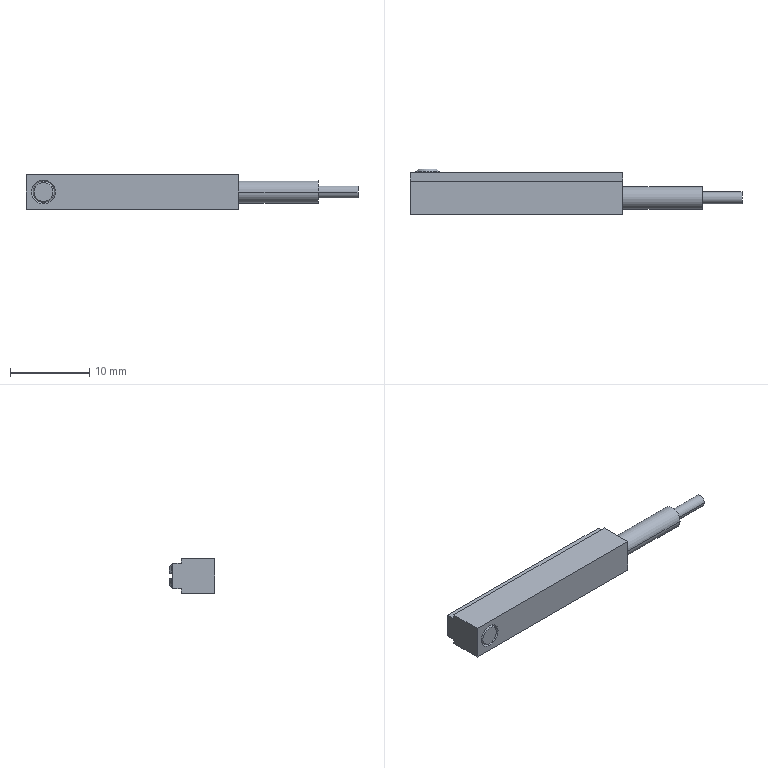Part | SolidWorks | features BaseBody 1 | 1 solid | 34 faces | box 41.8 x 5.7 x 4.4 mm | volume 661.389 mm3 | plane 20 | cylinder 7 | cone 7 | commonest cylinder face diameters 3 x3 1.5 x2 2.8 x2
STEP:
#1=CARTESIAN_POINT('',(2.2,3.2,-1.5));
#2=VERTEX_POINT('',#1);
#3=CARTESIAN_POINT('',(3.67,3.2,-0.3));
#4=VERTEX_POINT('',#3);
#5=CARTESIAN_POINT('',(2.2,3.2,0.));
#6=DIRECTION('',(0.,-1.,0.));
#7=DIRECTION('',(1.,0.,0.));
#8=AXIS2_PLACEMENT_3D('',#5,#6,#7);
#9=CIRCLE('',#8,1.5);
#10=EDGE_CURVE('',#2,#4,#9,.T.);
#11=ORIENTED_EDGE('',*,*,#10,.F.);
#12=CARTESIAN_POINT('',(2.2,3.293,-1.5));
#13=VERTEX_POINT('',#12);
#14=CARTESIAN_POINT('',(2.2,-2.1,-1.5));
#15=DIRECTION('',(0.,1.,0.));
#16=VECTOR('',#15,1000.);
#17=LINE('',#14,#16);
#18=EDGE_CURVE('',#2,#13,#17,.T.);
#19=ORIENTED_EDGE('',*,*,#18,.T.);
#20=CARTESIAN_POINT('',(3.67,3.293,-0.3));
#21=VERTEX_POINT('',#20);
#22=CARTESIAN_POINT('',(2.2,3.293,0.));
#23=DIRECTION('',(0.,-1.,0.));
#24=DIRECTION('',(0.,0.,-1.));
#25=AXIS2_PLACEMENT_3D('',#22,#23,#24);
#26=CIRCLE('',#25,1.5);
#27=EDGE_CURVE('',#13,#21,#26,.T.);
#28=ORIENTED_EDGE('',*,*,#27,.T.);
#29=CARTESIAN_POINT('',(3.67,-2.1,-0.3));
#30=DIRECTION('',(0.,1.,0.));
#31=VECTOR('',#30,1000.);
#32=LINE('',#29,#31);
#33=EDGE_CURVE('',#4,#21,#32,.T.);
#34=ORIENTED_EDGE('',*,*,#33,.F.);
#35=EDGE_LOOP('',(#11,#19,#28,#34));
#36=FACE_OUTER_BOUND('',#35,.T.);
#37=CARTESIAN_POINT('',(2.2,-2.1,0.));
#38=DIRECTION('',(0.,1.,0.));
#39=DIRECTION('',(0.,0.,-1.));
#40=AXIS2_PLACEMENT_3D('',#37,#38,#39);
#41=CYLINDRICAL_SURFACE('',#40,1.5);
#42=ADVANCED_FACE('',(#36),#41,.T.);
#43=CARTESIAN_POINT('',(1.045,3.6,-0.3));
#44=VERTEX_POINT('',#43);
#45=CARTESIAN_POINT('',(2.2,3.6,-1.194));
#46=VERTEX_POINT('',#45);
#47=CARTESIAN_POINT('',(2.2,3.6,0.));
#48=DIRECTION('',(0.,-1.,0.));
#49=DIRECTION('',(0.,0.,-1.));
#50=AXIS2_PLACEMENT_3D('',#47,#48,#49);
#51=CIRCLE('',#50,1.194);
#52=EDGE_CURVE('',#44,#46,#51,.T.);
#53=ORIENTED_EDGE('',*,*,#52,.T.);
#54=CARTESIAN_POINT('',(2.2,3.6,-1.194));
#55=DIRECTION('',(0.,-0.7071,-0.7071));
#56=VECTOR('',#55,1000.);
#57=LINE('',#54,#56);
#58=EDGE_CURVE('',#46,#13,#57,.T.);
#59=ORIENTED_EDGE('',*,*,#58,.T.);
#60=CARTESIAN_POINT('',(0.7303,3.293,-0.3));
#61=VERTEX_POINT('',#60);
#62=CARTESIAN_POINT('',(2.2,3.293,0.));
#63=DIRECTION('',(0.,-1.,0.));
#64=DIRECTION('',(0.,0.,-1.));
#65=AXIS2_PLACEMENT_3D('',#62,#63,#64);
#66=CIRCLE('',#65,1.5);
#67=EDGE_CURVE('',#61,#13,#66,.T.);
#68=ORIENTED_EDGE('',*,*,#67,.F.);
#69=CARTESIAN_POINT('',(1.045,3.6,-0.3));
#70=CARTESIAN_POINT('',(0.9396,3.498,-0.3));
#71=CARTESIAN_POINT('',(0.8349,3.396,-0.3));
#72=CARTESIAN_POINT('',(0.7303,3.293,-0.3));
#73=B_SPLINE_CURVE_WITH_KNOTS('',3,(#69,#70,#71,#72),.UNSPECIFIED.,.F.,.F.,(4,4),(0.005968,0.006407),.UNSPECIFIED.);
#74=EDGE_CURVE('',#44,#61,#73,.T.);
#75=ORIENTED_EDGE('',*,*,#74,.F.);
#76=EDGE_LOOP('',(#53,#59,#68,#75));
#77=FACE_OUTER_BOUND('',#76,.T.);
#78=CARTESIAN_POINT('',(2.2,3.6,0.));
#79=DIRECTION('',(0.,-1.,0.));
#80=DIRECTION('',(0.,0.,-1.));
#81=AXIS2_PLACEMENT_3D('',#78,#79,#80);
#82=CONICAL_SURFACE('',#81,1.194,0.7854);
#83=ADVANCED_FACE('',(#77),#82,.T.);
#84=CARTESIAN_POINT('',(36.8,-1.4,0.));
#85=VERTEX_POINT('',#84);
#86=CARTESIAN_POINT('',(36.8,1.4,0.));
#87=VERTEX_POINT('',#86);
#88=CARTESIAN_POINT('',(36.8,0.,0.));
#89=DIRECTION('',(1.,0.,0.));
#90=DIRECTION('',(0.,1.,0.));
#91=AXIS2_PLACEMENT_3D('',#88,#89,#90);
#92=CIRCLE('',#91,1.4);
#93=EDGE_CURVE('',#85,#87,#92,.T.);
#94=ORIENTED_EDGE('',*,*,#93,.F.);
#95=CARTESIAN_POINT('',(26.8,-1.4,0.));
#96=VERTEX_POINT('',#95);
#97=CARTESIAN_POINT('',(41.8,-1.4,0.));
#98=DIRECTION('',(-1.,0.,0.));
#99=VECTOR('',#98,1000.);
#100=LINE('',#97,#99);
#101=EDGE_CURVE('',#85,#96,#100,.T.);
#102=ORIENTED_EDGE('',*,*,#101,.T.);
#103=CARTESIAN_POINT('',(26.8,1.4,0.));
#104=VERTEX_POINT('',#103);
#105=CARTESIAN_POINT('',(26.8,0.,0.));
#106=DIRECTION('',(1.,0.,0.));
#107=DIRECTION('',(0.,1.,0.));
#108=AXIS2_PLACEMENT_3D('',#105,#106,#107);
#109=CIRCLE('',#108,1.4);
#110=EDGE_CURVE('',#96,#104,#109,.T.);
#111=ORIENTED_EDGE('',*,*,#110,.T.);
#112=CARTESIAN_POINT('',(41.8,1.4,0.));
#113=DIRECTION('',(-1.,0.,0.));
#114=VECTOR('',#113,1000.);
#115=LINE('',#112,#114);
#116=EDGE_CURVE('',#87,#104,#115,.T.);
#117=ORIENTED_EDGE('',*,*,#116,.F.);
#118=EDGE_LOOP('',(#94,#102,#111,#117));
#119=FACE_OUTER_BOUND('',#118,.T.);
#120=CARTESIAN_POINT('',(41.8,0.,0.));
#121=DIRECTION('',(-1.,0.,0.));
#122=DIRECTION('',(0.,1.,0.));
#123=AXIS2_PLACEMENT_3D('',#120,#121,#122);
#124=CYLINDRICAL_SURFACE('',#123,1.4);
#125=ADVANCED_FACE('',(#119),#124,.T.);
#126=CARTESIAN_POINT('',(41.8,-0.75,0.));
#127=VERTEX_POINT('',#126);
#128=CARTESIAN_POINT('',(41.8,0.75,0.));
#129=VERTEX_POINT('',#128);
#130=CARTESIAN_POINT('',(41.8,0.,0.));
#131=DIRECTION('',(1.,0.,0.));
#132=DIRECTION('',(0.,1.,0.));
#133=AXIS2_PLACEMENT_3D('',#130,#131,#132);
#134=CIRCLE('',#133,0.75);
#135=EDGE_CURVE('',#127,#129,#134,.T.);
#136=ORIENTED_EDGE('',*,*,#135,.F.);
#137=CARTESIAN_POINT('',(36.8,-0.75,0.));
#138=VERTEX_POINT('',#137);
#139=CARTESIAN_POINT('',(41.8,-0.75,0.));
#140=DIRECTION('',(-1.,0.,0.));
#141=VECTOR('',#140,1000.);
#142=LINE('',#139,#141);
#143=EDGE_CURVE('',#127,#138,#142,.T.);
#144=ORIENTED_EDGE('',*,*,#143,.T.);
#145=CARTESIAN_POINT('',(36.8,0.75,0.));
#146=VERTEX_POINT('',#145);
#147=CARTESIAN_POINT('',(36.8,0.,0.));
#148=DIRECTION('',(1.,0.,0.));
#149=DIRECTION('',(0.,1.,0.));
#150=AXIS2_PLACEMENT_3D('',#147,#148,#149);
#151=CIRCLE('',#150,0.75);
#152=EDGE_CURVE('',#138,#146,#151,.T.);
#153=ORIENTED_EDGE('',*,*,#152,.T.);
#154=CARTESIAN_POINT('',(41.8,0.75,0.));
#155=DIRECTION('',(-1.,0.,0.));
#156=VECTOR('',#155,1000.);
#157=LINE('',#154,#156);
#158=EDGE_CURVE('',#129,#146,#157,.T.);
#159=ORIENTED_EDGE('',*,*,#158,.F.);
#160=EDGE_LOOP('',(#136,#144,#153,#159));
#161=FACE_OUTER_BOUND('',#160,.T.);
#162=CARTESIAN_POINT('',(41.8,0.,0.));
#163=DIRECTION('',(-1.,0.,0.));
#164=DIRECTION('',(0.,1.,0.));
#165=AXIS2_PLACEMENT_3D('',#162,#163,#164);
#166=CYLINDRICAL_SURFACE('',#165,0.75);
#167=ADVANCED_FACE('',(#161),#166,.T.);
#168=CARTESIAN_POINT('',(2.2,-2.1,-1.194));
#169=VERTEX_POINT('',#168);
#170=CARTESIAN_POINT('',(2.2,-2.1,1.194));
#171=VERTEX_POINT('',#170);
#172=CARTESIAN_POINT('',(2.2,-2.1,0.));
#173=DIRECTION('',(0.,-1.,0.));
#174=DIRECTION('',(0.,0.,-1.));
#175=AXIS2_PLACEMENT_3D('',#172,#173,#174);
#176=CIRCLE('',#175,1.194);
#177=EDGE_CURVE('',#169,#171,#176,.T.);
#178=ORIENTED_EDGE('',*,*,#177,.F.);
#179=CARTESIAN_POINT('',(2.2,-1.947,-1.347));
#180=VERTEX_POINT('',#179);
#181=CARTESIAN_POINT('',(2.2,-1.793,-1.5));
#182=DIRECTION('',(0.,0.7071,-0.7071));
#183=VECTOR('',#182,1000.);
#184=LINE('',#181,#183);
#185=EDGE_CURVE('',#169,#180,#184,.T.);
#186=ORIENTED_EDGE('',*,*,#185,.T.);
#187=CARTESIAN_POINT('',(3.547,-1.947,0.));
#188=VERTEX_POINT('',#187);
#189=CARTESIAN_POINT('',(2.2,-1.947,0.));
#190=DIRECTION('',(0.,1.,0.));
#191=DIRECTION('',(0.,0.,1.));
#192=AXIS2_PLACEMENT_3D('',#189,#190,#191);
#193=CIRCLE('',#192,1.347);
#194=EDGE_CURVE('',#188,#180,#193,.T.);
#195=ORIENTED_EDGE('',*,*,#194,.F.);
#196=CARTESIAN_POINT('',(2.2,-1.947,1.347));
#197=VERTEX_POINT('',#196);
#198=CARTESIAN_POINT('',(2.2,-1.947,0.));
#199=DIRECTION('',(0.,1.,0.));
#200=DIRECTION('',(0.,0.,1.));
#201=AXIS2_PLACEMENT_3D('',#198,#199,#200);
#202=CIRCLE('',#201,1.347);
#203=EDGE_CURVE('',#197,#188,#202,.T.);
#204=ORIENTED_EDGE('',*,*,#203,.F.);
#205=CARTESIAN_POINT('',(2.2,-1.793,1.5));
#206=DIRECTION('',(0.,0.7071,0.7071));
#207=VECTOR('',#206,1000.);
#208=LINE('',#205,#207);
#209=EDGE_CURVE('',#171,#197,#208,.T.);
#210=ORIENTED_EDGE('',*,*,#209,.F.);
#211=EDGE_LOOP('',(#178,#186,#195,#204,#210));
#212=FACE_OUTER_BOUND('',#211,.T.);
#213=CARTESIAN_POINT('',(2.2,-1.793,0.));
#214=DIRECTION('',(0.,1.,0.));
#215=DIRECTION('',(0.,0.,1.));
#216=AXIS2_PLACEMENT_3D('',#213,#214,#215);
#217=CONICAL_SURFACE('',#216,1.5,0.7854);
#218=ADVANCED_FACE('',(#212),#217,.T.);
#219=ORIENTED_EDGE('',*,*,#194,.T.);
#220=CARTESIAN_POINT('',(0.8533,-1.947,0.));
#221=VERTEX_POINT('',#220);
#222=CARTESIAN_POINT('',(2.2,-1.947,0.));
#223=DIRECTION('',(0.,1.,0.));
#224=DIRECTION('',(0.,0.,1.));
#225=AXIS2_PLACEMENT_3D('',#222,#223,#224);
#226=CIRCLE('',#225,1.347);
#227=EDGE_CURVE('',#180,#221,#226,.T.);
#228=ORIENTED_EDGE('',*,*,#227,.T.);
#229=CARTESIAN_POINT('',(0.7,-2.1,0.));
#230=VERTEX_POINT('',#229);
#231=CARTESIAN_POINT('',(0.9705,-1.83,0.));
#232=DIRECTION('',(-0.7071,-0.7071,0.));
#233=VECTOR('',#232,1000.);
#234=LINE('',#231,#233);
#235=EDGE_CURVE('',#221,#230,#234,.T.);
#236=ORIENTED_EDGE('',*,*,#235,.T.);
#237=CARTESIAN_POINT('',(3.7,-2.1,0.));
#238=VERTEX_POINT('',#237);
#239=CARTESIAN_POINT('',(2.2,-2.1,0.));
#240=DIRECTION('',(0.,-1.,0.));
#241=DIRECTION('',(1.,0.,0.));
#242=AXIS2_PLACEMENT_3D('',#239,#240,#241);
#243=CIRCLE('',#242,1.5);
#244=EDGE_CURVE('',#230,#238,#243,.T.);
#245=ORIENTED_EDGE('',*,*,#244,.T.);
#246=CARTESIAN_POINT('',(3.43,-1.829,0.));
#247=DIRECTION('',(0.7071,-0.7071,0.));
#248=VECTOR('',#247,1000.);
#249=LINE('',#246,#248);
#250=EDGE_CURVE('',#188,#238,#249,.T.);
#251=ORIENTED_EDGE('',*,*,#250,.F.);
#252=EDGE_LOOP('',(#219,#228,#236,#245,#251));
#253=FACE_OUTER_BOUND('',#252,.T.);
#254=CARTESIAN_POINT('',(2.2,-1.829,0.));
#255=DIRECTION('',(0.,-1.,0.));
#256=DIRECTION('',(1.,0.,0.));
#257=AXIS2_PLACEMENT_3D('',#254,#255,#256);
#258=CONICAL_SURFACE('',#257,1.23,0.7854);
#259=ADVANCED_FACE('',(#253),#258,.F.);
#260=CARTESIAN_POINT('',(0.,-2.1,-2.2));
#261=VERTEX_POINT('',#260);
#262=CARTESIAN_POINT('',(0.,2.1,-2.2));
#263=VERTEX_POINT('',#262);
#264=CARTESIAN_POINT('',(0.,-2.1,-2.2));
#265=DIRECTION('',(0.,1.,0.));
#266=VECTOR('',#265,1000.);
#267=LINE('',#264,#266);
#268=EDGE_CURVE('',#261,#263,#267,.T.);
#269=ORIENTED_EDGE('',*,*,#268,.T.);
#270=CARTESIAN_POINT('',(26.8,2.1,-2.2));
#271=VERTEX_POINT('',#270);
#272=CARTESIAN_POINT('',(26.8,2.1,-2.2));
#273=DIRECTION('',(-1.,0.,0.));
#274=VECTOR('',#273,1000.);
#275=LINE('',#272,#274);
#276=EDGE_CURVE('',#271,#263,#275,.T.);
#277=ORIENTED_EDGE('',*,*,#276,.F.);
#278=CARTESIAN_POINT('',(26.8,-2.1,-2.2));
#279=VERTEX_POINT('',#278);
#280=CARTESIAN_POINT('',(26.8,-2.1,-2.2));
#281=DIRECTION('',(0.,1.,0.));
#282=VECTOR('',#281,1000.);
#283=LINE('',#280,#282);
#284=EDGE_CURVE('',#279,#271,#283,.T.);
#285=ORIENTED_EDGE('',*,*,#284,.F.);
#286=CARTESIAN_POINT('',(26.8,-2.1,-2.2));
#287=DIRECTION('',(-1.,0.,0.));
#288=VECTOR('',#287,1000.);
#289=LINE('',#286,#288);
#290=EDGE_CURVE('',#279,#261,#289,.T.);
#291=ORIENTED_EDGE('',*,*,#290,.T.);
#292=EDGE_LOOP('',(#269,#277,#285,#291));
#293=FACE_OUTER_BOUND('',#292,.T.);
#294=CARTESIAN_POINT('',(26.8,-2.1,-2.2));
#295=DIRECTION('',(0.,0.,1.));
#296=DIRECTION('',(1.,0.,0.));
#297=AXIS2_PLACEMENT_3D('',#294,#295,#296);
#298=PLANE('',#297);
#299=ADVANCED_FACE('',(#293),#298,.F.);
#300=CARTESIAN_POINT('',(0.,2.1,-1.6));
#301=VERTEX_POINT('',#300);
#302=CARTESIAN_POINT('',(0.,2.1,-2.2));
#303=DIRECTION('',(0.,0.,1.));
#304=VECTOR('',#303,1000.);
#305=LINE('',#302,#304);
#306=EDGE_CURVE('',#263,#301,#305,.T.);
#307=ORIENTED_EDGE('',*,*,#306,.T.);
#308=CARTESIAN_POINT('',(26.8,2.1,-1.6));
#309=VERTEX_POINT('',#308);
#310=CARTESIAN_POINT('',(26.8,2.1,-1.6));
#311=DIRECTION('',(-1.,0.,0.));
#312=VECTOR('',#311,1000.);
#313=LINE('',#310,#312);
#314=EDGE_CURVE('',#309,#301,#313,.T.);
#315=ORIENTED_EDGE('',*,*,#314,.F.);
#316=CARTESIAN_POINT('',(26.8,2.1,-2.2));
#317=DIRECTION('',(0.,0.,1.));
#318=VECTOR('',#317,1000.);
#319=LINE('',#316,#318);
#320=EDGE_CURVE('',#271,#309,#319,.T.);
#321=ORIENTED_EDGE('',*,*,#320,.F.);
#322=ORIENTED_EDGE('',*,*,#276,.T.);
#323=EDGE_LOOP('',(#307,#315,#321,#322));
#324=FACE_OUTER_BOUND('',#323,.T.);
#325=CARTESIAN_POINT('',(26.8,2.1,-2.2));
#326=DIRECTION('',(0.,-1.,0.));
#327=DIRECTION('',(0.,0.,-1.));
#328=AXIS2_PLACEMENT_3D('',#325,#326,#327);
#329=PLANE('',#328);
#330=ADVANCED_FACE('',(#324),#329,.F.);
#331=CARTESIAN_POINT('',(0.,-2.1,2.2));
#332=VERTEX_POINT('',#331);
#333=CARTESIAN_POINT('',(0.,-2.1,2.2));
#334=DIRECTION('',(0.,0.,-1.));
#335=VECTOR('',#334,1000.);
#336=LINE('',#333,#335);
#337=EDGE_CURVE('',#332,#261,#336,.T.);
#338=ORIENTED_EDGE('',*,*,#337,.T.);
#339=ORIENTED_EDGE('',*,*,#290,.F.);
#340=CARTESIAN_POINT('',(26.8,-2.1,2.2));
#341=VERTEX_POINT('',#340);
#342=CARTESIAN_POINT('',(26.8,-2.1,2.2));
#343=DIRECTION('',(0.,0.,-1.));
#344=VECTOR('',#343,1000.);
#345=LINE('',#342,#344);
#346=EDGE_CURVE('',#341,#279,#345,.T.);
#347=ORIENTED_EDGE('',*,*,#346,.F.);
#348=CARTESIAN_POINT('',(26.8,-2.1,2.2));
#349=DIRECTION('',(-1.,0.,0.));
#350=VECTOR('',#349,1000.);
#351=LINE('',#348,#350);
#352=EDGE_CURVE('',#341,#332,#351,.T.);
#353=ORIENTED_EDGE('',*,*,#352,.T.);
#354=EDGE_LOOP('',(#338,#339,#347,#353));
#355=FACE_OUTER_BOUND('',#354,.T.);
#356=CARTESIAN_POINT('',(2.2,-2.1,0.));
#357=DIRECTION('',(0.,-1.,0.));
#358=DIRECTION('',(1.,0.,0.));
#359=AXIS2_PLACEMENT_3D('',#356,#357,#358);
#360=CIRCLE('',#359,1.5);
#361=EDGE_CURVE('',#238,#230,#360,.T.);
#362=ORIENTED_EDGE('',*,*,#361,.F.);
#363=ORIENTED_EDGE('',*,*,#244,.F.);
#364=EDGE_LOOP('',(#362,#363));
#365=FACE_BOUND('',#364,.T.);
#366=CARTESIAN_POINT('',(26.8,-2.1,2.2));
#367=DIRECTION('',(0.,1.,0.));
#368=DIRECTION('',(1.,0.,0.));
#369=AXIS2_PLACEMENT_3D('',#366,#367,#368);
#370=PLANE('',#369);
#371=ADVANCED_FACE('',(#355,#365),#370,.F.);
#372=CARTESIAN_POINT('',(0.,3.2,-1.6));
#373=VERTEX_POINT('',#372);
#374=CARTESIAN_POINT('',(0.,3.2,1.6));
#375=VERTEX_POINT('',#374);
#376=CARTESIAN_POINT('',(0.,3.2,-1.6));
#377=DIRECTION('',(0.,0.,1.));
#378=VECTOR('',#377,1000.);
#379=LINE('',#376,#378);
#380=EDGE_CURVE('',#373,#375,#379,.T.);
#381=ORIENTED_EDGE('',*,*,#380,.T.);
#382=CARTESIAN_POINT('',(26.8,3.2,1.6));
#383=VERTEX_POINT('',#382);
#384=CARTESIAN_POINT('',(26.8,3.2,1.6));
#385=DIRECTION('',(-1.,0.,0.));
#386=VECTOR('',#385,1000.);
#387=LINE('',#384,#386);
#388=EDGE_CURVE('',#383,#375,#387,.T.);
#389=ORIENTED_EDGE('',*,*,#388,.F.);
#390=CARTESIAN_POINT('',(26.8,3.2,-1.6));
#391=VERTEX_POINT('',#390);
#392=CARTESIAN_POINT('',(26.8,3.2,-1.6));
#393=DIRECTION('',(0.,0.,1.));
#394=VECTOR('',#393,1000.);
#395=LINE('',#392,#394);
#396=EDGE_CURVE('',#391,#383,#395,.T.);
#397=ORIENTED_EDGE('',*,*,#396,.F.);
#398=CARTESIAN_POINT('',(26.8,3.2,-1.6));
#399=DIRECTION('',(-1.,0.,0.));
#400=VECTOR('',#399,1000.);
#401=LINE('',#398,#400);
#402=EDGE_CURVE('',#391,#373,#401,.T.);
#403=ORIENTED_EDGE('',*,*,#402,.T.);
#404=EDGE_LOOP('',(#381,#389,#397,#403));
#405=FACE_OUTER_BOUND('',#404,.T.);
#406=CARTESIAN_POINT('',(3.7,3.2,0.3));
#407=VERTEX_POINT('',#406);
#408=CARTESIAN_POINT('',(3.7,3.2,-0.3));
#409=VERTEX_POINT('',#408);
#410=CARTESIAN_POINT('',(3.7,3.2,-1.6));
#411=DIRECTION('',(0.,0.,-1.));
#412=VECTOR('',#411,1000.);
#413=LINE('',#410,#412);
#414=EDGE_CURVE('',#407,#409,#413,.T.);
#415=ORIENTED_EDGE('',*,*,#414,.F.);
#416=CARTESIAN_POINT('',(3.67,3.2,0.3));
#417=VERTEX_POINT('',#416);
#418=CARTESIAN_POINT('',(26.8,3.2,0.3));
#419=DIRECTION('',(-1.,0.,0.));
#420=VECTOR('',#419,1000.);
#421=LINE('',#418,#420);
#422=EDGE_CURVE('',#407,#417,#421,.T.);
#423=ORIENTED_EDGE('',*,*,#422,.T.);
#424=CARTESIAN_POINT('',(0.7303,3.2,0.3));
#425=VERTEX_POINT('',#424);
#426=CARTESIAN_POINT('',(2.2,3.2,0.));
#427=DIRECTION('',(0.,-1.,0.));
#428=DIRECTION('',(1.,0.,0.));
#429=AXIS2_PLACEMENT_3D('',#426,#427,#428);
#430=CIRCLE('',#429,1.5);
#431=EDGE_CURVE('',#417,#425,#430,.T.);
#432=ORIENTED_EDGE('',*,*,#431,.T.);
#433=CARTESIAN_POINT('',(0.7,3.2,0.3));
#434=VERTEX_POINT('',#433);
#435=CARTESIAN_POINT('',(26.8,3.2,0.3));
#436=DIRECTION('',(-1.,0.,0.));
#437=VECTOR('',#436,1000.);
#438=LINE('',#435,#437);
#439=EDGE_CURVE('',#425,#434,#438,.T.);
#440=ORIENTED_EDGE('',*,*,#439,.T.);
#441=CARTESIAN_POINT('',(0.7,3.2,-0.3));
#442=VERTEX_POINT('',#441);
#443=CARTESIAN_POINT('',(0.7,3.2,-1.6));
#444=DIRECTION('',(0.,0.,1.));
#445=VECTOR('',#444,1000.);
#446=LINE('',#443,#445);
#447=EDGE_CURVE('',#442,#434,#446,.T.);
#448=ORIENTED_EDGE('',*,*,#447,.F.);
#449=CARTESIAN_POINT('',(0.7303,3.2,-0.3));
#450=VERTEX_POINT('',#449);
#451=CARTESIAN_POINT('',(26.8,3.2,-0.3));
#452=DIRECTION('',(-1.,0.,0.));
#453=VECTOR('',#452,1000.);
#454=LINE('',#451,#453);
#455=EDGE_CURVE('',#450,#442,#454,.T.);
#456=ORIENTED_EDGE('',*,*,#455,.F.);
#457=CARTESIAN_POINT('',(2.2,3.2,0.));
#458=DIRECTION('',(0.,-1.,0.));
#459=DIRECTION('',(1.,0.,0.));
#460=AXIS2_PLACEMENT_3D('',#457,#458,#459);
#461=CIRCLE('',#460,1.5);
#462=EDGE_CURVE('',#450,#2,#461,.T.);
#463=ORIENTED_EDGE('',*,*,#462,.T.);
#464=ORIENTED_EDGE('',*,*,#10,.T.);
#465=CARTESIAN_POINT('',(26.8,3.2,-0.3));
#466=DIRECTION('',(-1.,0.,0.));
#467=VECTOR('',#466,1000.);
#468=LINE('',#465,#467);
#469=EDGE_CURVE('',#409,#4,#468,.T.);
#470=ORIENTED_EDGE('',*,*,#469,.F.);
#471=EDGE_LOOP('',(#415,#423,#432,#440,#448,#456,#463,#464,#470));
#472=FACE_BOUND('',#471,.T.);
#473=CARTESIAN_POINT('',(26.8,3.2,-1.6));
#474=DIRECTION('',(0.,-1.,0.));
#475=DIRECTION('',(0.,0.,-1.));
#476=AXIS2_PLACEMENT_3D('',#473,#474,#475);
#477=PLANE('',#476);
#478=ADVANCED_FACE('',(#405,#472),#477,.F.);
#479=CARTESIAN_POINT('',(3.355,3.6,-0.3));
#480=VERTEX_POINT('',#479);
#481=CARTESIAN_POINT('',(3.7,3.6,-0.3));
#482=DIRECTION('',(-1.,0.,0.));
#483=VECTOR('',#482,1000.);
#484=LINE('',#481,#483);
#485=EDGE_CURVE('',#480,#44,#484,.T.);
#486=ORIENTED_EDGE('',*,*,#485,.F.);
#487=CARTESIAN_POINT('',(2.2,3.6,0.));
#488=DIRECTION('',(0.,-1.,0.));
#489=DIRECTION('',(0.,0.,-1.));
#490=AXIS2_PLACEMENT_3D('',#487,#488,#489);
#491=CIRCLE('',#490,1.194);
#492=EDGE_CURVE('',#46,#480,#491,.T.);
#493=ORIENTED_EDGE('',*,*,#492,.F.);
#494=ORIENTED_EDGE('',*,*,#52,.F.);
#495=EDGE_LOOP('',(#486,#493,#494));
#496=FACE_OUTER_BOUND('',#495,.T.);
#497=CARTESIAN_POINT('',(2.2,3.6,0.));
#498=DIRECTION('',(0.,-1.,0.));
#499=DIRECTION('',(0.,0.,-1.));
#500=AXIS2_PLACEMENT_3D('',#497,#498,#499);
#501=PLANE('',#500);
#502=ADVANCED_FACE('',(#496),#501,.F.);
#503=CARTESIAN_POINT('',(0.,2.1,-1.6));
#504=DIRECTION('',(0.,1.,0.));
#505=VECTOR('',#504,1000.);
#506=LINE('',#503,#505);
#507=EDGE_CURVE('',#301,#373,#506,.T.);
#508=ORIENTED_EDGE('',*,*,#507,.T.);
#509=ORIENTED_EDGE('',*,*,#402,.F.);
#510=CARTESIAN_POINT('',(26.8,2.1,-1.6));
#511=DIRECTION('',(0.,1.,0.));
#512=VECTOR('',#511,1000.);
#513=LINE('',#510,#512);
#514=EDGE_CURVE('',#309,#391,#513,.T.);
#515=ORIENTED_EDGE('',*,*,#514,.F.);
#516=ORIENTED_EDGE('',*,*,#314,.T.);
#517=EDGE_LOOP('',(#508,#509,#515,#516));
#518=FACE_OUTER_BOUND('',#517,.T.);
#519=CARTESIAN_POINT('',(26.8,2.1,-1.6));
#520=DIRECTION('',(0.,0.,1.));
#521=DIRECTION('',(1.,0.,0.));
#522=AXIS2_PLACEMENT_3D('',#519,#520,#521);
#523=PLANE('',#522);
#524=ADVANCED_FACE('',(#518),#523,.F.);
#525=CARTESIAN_POINT('',(0.,2.1,1.6));
#526=VERTEX_POINT('',#525);
#527=CARTESIAN_POINT('',(0.,3.2,1.6));
#528=DIRECTION('',(0.,-1.,0.));
#529=VECTOR('',#528,1000.);
#530=LINE('',#527,#529);
#531=EDGE_CURVE('',#375,#526,#530,.T.);
#532=ORIENTED_EDGE('',*,*,#531,.T.);
#533=CARTESIAN_POINT('',(26.8,2.1,1.6));
#534=VERTEX_POINT('',#533);
#535=CARTESIAN_POINT('',(26.8,2.1,1.6));
#536=DIRECTION('',(-1.,0.,0.));
#537=VECTOR('',#536,1000.);
#538=LINE('',#535,#537);
#539=EDGE_CURVE('',#534,#526,#538,.T.);
#540=ORIENTED_EDGE('',*,*,#539,.F.);
#541=CARTESIAN_POINT('',(26.8,3.2,1.6));
#542=DIRECTION('',(0.,-1.,0.));
#543=VECTOR('',#542,1000.);
#544=LINE('',#541,#543);
#545=EDGE_CURVE('',#383,#534,#544,.T.);
#546=ORIENTED_EDGE('',*,*,#545,.F.);
#547=ORIENTED_EDGE('',*,*,#388,.T.);
#548=EDGE_LOOP('',(#532,#540,#546,#547));
#549=FACE_OUTER_BOUND('',#548,.T.);
#550=CARTESIAN_POINT('',(26.8,3.2,1.6));
#551=DIRECTION('',(0.,0.,-1.));
#552=DIRECTION('',(0.,-1.,0.));
#553=AXIS2_PLACEMENT_3D('',#550,#551,#552);
#554=PLANE('',#553);
#555=ADVANCED_FACE('',(#549),#554,.F.);
#556=CARTESIAN_POINT('',(0.,2.1,2.2));
#557=VERTEX_POINT('',#556);
#558=CARTESIAN_POINT('',(0.,2.1,1.6));
#559=DIRECTION('',(0.,0.,1.));
#560=VECTOR('',#559,1000.);
#561=LINE('',#558,#560);
#562=EDGE_CURVE('',#526,#557,#561,.T.);
#563=ORIENTED_EDGE('',*,*,#562,.T.);
#564=CARTESIAN_POINT('',(26.8,2.1,2.2));
#565=VERTEX_POINT('',#564);
#566=CARTESIAN_POINT('',(26.8,2.1,2.2));
#567=DIRECTION('',(-1.,0.,0.));
#568=VECTOR('',#567,1000.);
#569=LINE('',#566,#568);
#570=EDGE_CURVE('',#565,#557,#569,.T.);
#571=ORIENTED_EDGE('',*,*,#570,.F.);
#572=CARTESIAN_POINT('',(26.8,2.1,1.6));
#573=DIRECTION('',(0.,0.,1.));
#574=VECTOR('',#573,1000.);
#575=LINE('',#572,#574);
#576=EDGE_CURVE('',#534,#565,#575,.T.);
#577=ORIENTED_EDGE('',*,*,#576,.F.);
#578=ORIENTED_EDGE('',*,*,#539,.T.);
#579=EDGE_LOOP('',(#563,#571,#577,#578));
#580=FACE_OUTER_BOUND('',#579,.T.);
#581=CARTESIAN_POINT('',(26.8,2.1,1.6));
#582=DIRECTION('',(0.,-1.,0.));
#583=DIRECTION('',(0.,0.,-1.));
#584=AXIS2_PLACEMENT_3D('',#581,#582,#583);
#585=PLANE('',#584);
#586=ADVANCED_FACE('',(#580),#585,.F.);
#587=CARTESIAN_POINT('',(26.8,2.1,2.2));
#588=DIRECTION('',(0.,-1.,0.));
#589=VECTOR('',#588,1000.);
#590=LINE('',#587,#589);
#591=EDGE_CURVE('',#565,#341,#590,.T.);
#592=ORIENTED_EDGE('',*,*,#591,.T.);
#593=ORIENTED_EDGE('',*,*,#346,.T.);
#594=ORIENTED_EDGE('',*,*,#284,.T.);
#595=ORIENTED_EDGE('',*,*,#320,.T.);
#596=ORIENTED_EDGE('',*,*,#514,.T.);
#597=ORIENTED_EDGE('',*,*,#396,.T.);
#598=ORIENTED_EDGE('',*,*,#545,.T.);
#599=ORIENTED_EDGE('',*,*,#576,.T.);
#600=EDGE_LOOP('',(#592,#593,#594,#595,#596,#597,#598,#599));
#601=FACE_OUTER_BOUND('',#600,.T.);
#602=CARTESIAN_POINT('',(26.8,0.,0.));
#603=DIRECTION('',(1.,0.,0.));
#604=DIRECTION('',(0.,1.,0.));
#605=AXIS2_PLACEMENT_3D('',#602,#603,#604);
#606=CIRCLE('',#605,1.4);
#607=EDGE_CURVE('',#104,#96,#606,.T.);
#608=ORIENTED_EDGE('',*,*,#607,.F.);
#609=ORIENTED_EDGE('',*,*,#110,.F.);
#610=EDGE_LOOP('',(#608,#609));
#611=FACE_BOUND('',#610,.T.);
#612=CARTESIAN_POINT('',(26.8,0.,0.));
#613=DIRECTION('',(1.,0.,0.));
#614=DIRECTION('',(0.,1.,0.));
#615=AXIS2_PLACEMENT_3D('',#612,#613,#614);
#616=PLANE('',#615);
#617=ADVANCED_FACE('',(#601,#611),#616,.T.);
#618=CARTESIAN_POINT('',(0.,2.1,2.2));
#619=DIRECTION('',(0.,-1.,0.));
#620=VECTOR('',#619,1000.);
#621=LINE('',#618,#620);
#622=EDGE_CURVE('',#557,#332,#621,.T.);
#623=ORIENTED_EDGE('',*,*,#622,.F.);
#624=ORIENTED_EDGE('',*,*,#562,.F.);
#625=ORIENTED_EDGE('',*,*,#531,.F.);
#626=ORIENTED_EDGE('',*,*,#380,.F.);
#627=ORIENTED_EDGE('',*,*,#507,.F.);
#628=ORIENTED_EDGE('',*,*,#306,.F.);
#629=ORIENTED_EDGE('',*,*,#268,.F.);
#630=ORIENTED_EDGE('',*,*,#337,.F.);
#631=EDGE_LOOP('',(#623,#624,#625,#626,#627,#628,#629,#630));
#632=FACE_OUTER_BOUND('',#631,.T.);
#633=CARTESIAN_POINT('',(0.,0.,0.));
#634=DIRECTION('',(1.,0.,0.));
#635=DIRECTION('',(0.,1.,0.));
#636=AXIS2_PLACEMENT_3D('',#633,#634,#635);
#637=PLANE('',#636);
#638=ADVANCED_FACE('',(#632),#637,.F.);
#639=ORIENTED_EDGE('',*,*,#235,.F.);
#640=CARTESIAN_POINT('',(2.2,-1.947,0.));
#641=DIRECTION('',(0.,1.,0.));
#642=DIRECTION('',(0.,0.,1.));
#643=AXIS2_PLACEMENT_3D('',#640,#641,#642);
#644=CIRCLE('',#643,1.347);
#645=EDGE_CURVE('',#221,#197,#644,.T.);
#646=ORIENTED_EDGE('',*,*,#645,.T.);
#647=ORIENTED_EDGE('',*,*,#203,.T.);
#648=ORIENTED_EDGE('',*,*,#250,.T.);
#649=ORIENTED_EDGE('',*,*,#361,.T.);
#650=EDGE_LOOP('',(#639,#646,#647,#648,#649));
#651=FACE_OUTER_BOUND('',#650,.T.);
#652=CARTESIAN_POINT('',(2.2,-1.829,0.));
#653=DIRECTION('',(0.,-1.,0.));
#654=DIRECTION('',(1.,0.,0.));
#655=AXIS2_PLACEMENT_3D('',#652,#653,#654);
#656=CONICAL_SURFACE('',#655,1.23,0.7854);
#657=ADVANCED_FACE('',(#651),#656,.F.);
#658=CARTESIAN_POINT('',(3.355,3.6,0.3));
#659=VERTEX_POINT('',#658);
#660=CARTESIAN_POINT('',(1.045,3.6,0.3));
#661=VERTEX_POINT('',#660);
#662=CARTESIAN_POINT('',(2.2,3.6,0.));
#663=DIRECTION('',(0.,-1.,0.));
#664=DIRECTION('',(0.,0.,-1.));
#665=AXIS2_PLACEMENT_3D('',#662,#663,#664);
#666=CIRCLE('',#665,1.194);
#667=EDGE_CURVE('',#659,#661,#666,.T.);
#668=ORIENTED_EDGE('',*,*,#667,.F.);
#669=CARTESIAN_POINT('',(3.7,3.6,0.3));
#670=DIRECTION('',(-1.,0.,0.));
#671=VECTOR('',#670,1000.);
#672=LINE('',#669,#671);
#673=EDGE_CURVE('',#659,#661,#672,.T.);
#674=ORIENTED_EDGE('',*,*,#673,.T.);
#675=EDGE_LOOP('',(#668,#674));
#676=FACE_OUTER_BOUND('',#675,.T.);
#677=CARTESIAN_POINT('',(2.2,3.6,0.));
#678=DIRECTION('',(0.,-1.,0.));
#679=DIRECTION('',(0.,0.,-1.));
#680=AXIS2_PLACEMENT_3D('',#677,#678,#679);
#681=PLANE('',#680);
#682=ADVANCED_FACE('',(#676),#681,.F.);
#683=CARTESIAN_POINT('',(3.67,3.293,0.3));
#684=VERTEX_POINT('',#683);
#685=CARTESIAN_POINT('',(0.7303,3.293,0.3));
#686=VERTEX_POINT('',#685);
#687=CARTESIAN_POINT('',(2.2,3.293,0.));
#688=DIRECTION('',(0.,-1.,0.));
#689=DIRECTION('',(0.,0.,-1.));
#690=AXIS2_PLACEMENT_3D('',#687,#688,#689);
#691=CIRCLE('',#690,1.5);
#692=EDGE_CURVE('',#684,#686,#691,.T.);
#693=ORIENTED_EDGE('',*,*,#692,.F.);
#694=CARTESIAN_POINT('',(3.67,3.293,0.3));
#695=CARTESIAN_POINT('',(3.565,3.396,0.3));
#696=CARTESIAN_POINT('',(3.46,3.498,0.3));
#697=CARTESIAN_POINT('',(3.355,3.6,0.3));
#698=B_SPLINE_CURVE_WITH_KNOTS('',3,(#694,#695,#696,#697),.UNSPECIFIED.,.F.,.F.,(4,4),(0.002571,0.00301),.UNSPECIFIED.);
#699=EDGE_CURVE('',#684,#659,#698,.T.);
#700=ORIENTED_EDGE('',*,*,#699,.T.);
#701=ORIENTED_EDGE('',*,*,#667,.T.);
#702=CARTESIAN_POINT('',(1.045,3.6,0.3));
#703=CARTESIAN_POINT('',(0.9396,3.498,0.3));
#704=CARTESIAN_POINT('',(0.8349,3.396,0.3));
#705=CARTESIAN_POINT('',(0.7303,3.293,0.3));
#706=B_SPLINE_CURVE_WITH_KNOTS('',3,(#702,#703,#704,#705),.UNSPECIFIED.,.F.,.F.,(4,4),(0.005968,0.006407),.UNSPECIFIED.);
#707=EDGE_CURVE('',#661,#686,#706,.T.);
#708=ORIENTED_EDGE('',*,*,#707,.T.);
#709=EDGE_LOOP('',(#693,#700,#701,#708));
#710=FACE_OUTER_BOUND('',#709,.T.);
#711=CARTESIAN_POINT('',(2.2,3.6,0.));
#712=DIRECTION('',(0.,-1.,0.));
#713=DIRECTION('',(0.,0.,-1.));
#714=AXIS2_PLACEMENT_3D('',#711,#712,#713);
#715=CONICAL_SURFACE('',#714,1.194,0.7854);
#716=ADVANCED_FACE('',(#710),#715,.T.);
#717=CARTESIAN_POINT('',(0.7303,-2.1,0.3));
#718=DIRECTION('',(0.,-1.,0.));
#719=VECTOR('',#718,1000.);
#720=LINE('',#717,#719);
#721=EDGE_CURVE('',#686,#425,#720,.T.);
#722=ORIENTED_EDGE('',*,*,#721,.F.);
#723=ORIENTED_EDGE('',*,*,#707,.F.);
#724=ORIENTED_EDGE('',*,*,#673,.F.);
#725=ORIENTED_EDGE('',*,*,#699,.F.);
#726=CARTESIAN_POINT('',(3.67,-2.1,0.3));
#727=DIRECTION('',(0.,1.,0.));
#728=VECTOR('',#727,1000.);
#729=LINE('',#726,#728);
#730=EDGE_CURVE('',#417,#684,#729,.T.);
#731=ORIENTED_EDGE('',*,*,#730,.F.);
#732=ORIENTED_EDGE('',*,*,#422,.F.);
#733=CARTESIAN_POINT('',(3.7,3.1,0.3));
#734=VERTEX_POINT('',#733);
#735=CARTESIAN_POINT('',(3.7,3.1,0.3));
#736=DIRECTION('',(0.,1.,0.));
#737=VECTOR('',#736,1000.);
#738=LINE('',#735,#737);
#739=EDGE_CURVE('',#734,#407,#738,.T.);
#740=ORIENTED_EDGE('',*,*,#739,.F.);
#741=CARTESIAN_POINT('',(0.7,3.1,0.3));
#742=VERTEX_POINT('',#741);
#743=CARTESIAN_POINT('',(0.7,3.1,0.3));
#744=DIRECTION('',(1.,0.,0.));
#745=VECTOR('',#744,1000.);
#746=LINE('',#743,#745);
#747=EDGE_CURVE('',#742,#734,#746,.T.);
#748=ORIENTED_EDGE('',*,*,#747,.F.);
#749=CARTESIAN_POINT('',(0.7,3.6,0.3));
#750=DIRECTION('',(0.,-1.,0.));
#751=VECTOR('',#750,1000.);
#752=LINE('',#749,#751);
#753=EDGE_CURVE('',#434,#742,#752,.T.);
#754=ORIENTED_EDGE('',*,*,#753,.F.);
#755=ORIENTED_EDGE('',*,*,#439,.F.);
#756=EDGE_LOOP('',(#722,#723,#724,#725,#731,#732,#740,#748,#754,#755));
#757=FACE_OUTER_BOUND('',#756,.T.);
#758=CARTESIAN_POINT('',(0.,0.,0.3));
#759=DIRECTION('',(0.,0.,1.));
#760=DIRECTION('',(1.,0.,0.));
#761=AXIS2_PLACEMENT_3D('',#758,#759,#760);
#762=PLANE('',#761);
#763=ADVANCED_FACE('',(#757),#762,.F.);
#764=ORIENTED_EDGE('',*,*,#455,.T.);
#765=CARTESIAN_POINT('',(0.7,3.1,-0.3));
#766=VERTEX_POINT('',#765);
#767=CARTESIAN_POINT('',(0.7,3.6,-0.3));
#768=DIRECTION('',(0.,-1.,0.));
#769=VECTOR('',#768,1000.);
#770=LINE('',#767,#769);
#771=EDGE_CURVE('',#442,#766,#770,.T.);
#772=ORIENTED_EDGE('',*,*,#771,.T.);
#773=CARTESIAN_POINT('',(3.7,3.1,-0.3));
#774=VERTEX_POINT('',#773);
#775=CARTESIAN_POINT('',(0.7,3.1,-0.3));
#776=DIRECTION('',(1.,0.,0.));
#777=VECTOR('',#776,1000.);
#778=LINE('',#775,#777);
#779=EDGE_CURVE('',#766,#774,#778,.T.);
#780=ORIENTED_EDGE('',*,*,#779,.T.);
#781=CARTESIAN_POINT('',(3.7,3.1,-0.3));
#782=DIRECTION('',(0.,1.,0.));
#783=VECTOR('',#782,1000.);
#784=LINE('',#781,#783);
#785=EDGE_CURVE('',#774,#409,#784,.T.);
#786=ORIENTED_EDGE('',*,*,#785,.T.);
#787=ORIENTED_EDGE('',*,*,#469,.T.);
#788=ORIENTED_EDGE('',*,*,#33,.T.);
#789=CARTESIAN_POINT('',(3.67,3.293,-0.3));
#790=CARTESIAN_POINT('',(3.565,3.396,-0.3));
#791=CARTESIAN_POINT('',(3.46,3.498,-0.3));
#792=CARTESIAN_POINT('',(3.355,3.6,-0.3));
#793=B_SPLINE_CURVE_WITH_KNOTS('',3,(#789,#790,#791,#792),.UNSPECIFIED.,.F.,.F.,(4,4),(0.002571,0.00301),.UNSPECIFIED.);
#794=EDGE_CURVE('',#21,#480,#793,.T.);
#795=ORIENTED_EDGE('',*,*,#794,.T.);
#796=ORIENTED_EDGE('',*,*,#485,.T.);
#797=ORIENTED_EDGE('',*,*,#74,.T.);
#798=CARTESIAN_POINT('',(0.7303,-2.1,-0.3));
#799=DIRECTION('',(0.,-1.,0.));
#800=VECTOR('',#799,1000.);
#801=LINE('',#798,#800);
#802=EDGE_CURVE('',#61,#450,#801,.T.);
#803=ORIENTED_EDGE('',*,*,#802,.T.);
#804=EDGE_LOOP('',(#764,#772,#780,#786,#787,#788,#795,#796,#797,#803));
#805=FACE_OUTER_BOUND('',#804,.T.);
#806=CARTESIAN_POINT('',(0.,0.,-0.3));
#807=DIRECTION('',(0.,0.,1.));
#808=DIRECTION('',(1.,0.,0.));
#809=AXIS2_PLACEMENT_3D('',#806,#807,#808);
#810=PLANE('',#809);
#811=ADVANCED_FACE('',(#805),#810,.T.);
#812=ORIENTED_EDGE('',*,*,#414,.T.);
#813=ORIENTED_EDGE('',*,*,#785,.F.);
#814=CARTESIAN_POINT('',(3.7,3.1,0.3));
#815=DIRECTION('',(0.,0.,-1.));
#816=VECTOR('',#815,1000.);
#817=LINE('',#814,#816);
#818=EDGE_CURVE('',#734,#774,#817,.T.);
#819=ORIENTED_EDGE('',*,*,#818,.F.);
#820=ORIENTED_EDGE('',*,*,#739,.T.);
#821=EDGE_LOOP('',(#812,#813,#819,#820));
#822=FACE_OUTER_BOUND('',#821,.T.);
#823=CARTESIAN_POINT('',(3.7,3.1,0.3));
#824=DIRECTION('',(-1.,0.,0.));
#825=DIRECTION('',(0.,0.,1.));
#826=AXIS2_PLACEMENT_3D('',#823,#824,#825);
#827=PLANE('',#826);
#828=ADVANCED_FACE('',(#822),#827,.T.);
#829=ORIENTED_EDGE('',*,*,#779,.F.);
#830=CARTESIAN_POINT('',(0.7,3.1,0.3));
#831=DIRECTION('',(0.,0.,-1.));
#832=VECTOR('',#831,1000.);
#833=LINE('',#830,#832);
#834=EDGE_CURVE('',#742,#766,#833,.T.);
#835=ORIENTED_EDGE('',*,*,#834,.F.);
#836=ORIENTED_EDGE('',*,*,#747,.T.);
#837=ORIENTED_EDGE('',*,*,#818,.T.);
#838=EDGE_LOOP('',(#829,#835,#836,#837));
#839=FACE_OUTER_BOUND('',#838,.T.);
#840=CARTESIAN_POINT('',(0.7,3.1,0.3));
#841=DIRECTION('',(0.,1.,0.));
#842=DIRECTION('',(1.,0.,0.));
#843=AXIS2_PLACEMENT_3D('',#840,#841,#842);
#844=PLANE('',#843);
#845=ADVANCED_FACE('',(#839),#844,.T.);
#846=ORIENTED_EDGE('',*,*,#447,.T.);
#847=ORIENTED_EDGE('',*,*,#753,.T.);
#848=ORIENTED_EDGE('',*,*,#834,.T.);
#849=ORIENTED_EDGE('',*,*,#771,.F.);
#850=EDGE_LOOP('',(#846,#847,#848,#849));
#851=FACE_OUTER_BOUND('',#850,.T.);
#852=CARTESIAN_POINT('',(0.7,3.6,0.3));
#853=DIRECTION('',(1.,0.,0.));
#854=DIRECTION('',(0.,1.,0.));
#855=AXIS2_PLACEMENT_3D('',#852,#853,#854);
#856=PLANE('',#855);
#857=ADVANCED_FACE('',(#851),#856,.T.);
#858=CARTESIAN_POINT('',(2.2,-2.1,0.));
#859=DIRECTION('',(0.,-1.,0.));
#860=DIRECTION('',(0.,0.,-1.));
#861=AXIS2_PLACEMENT_3D('',#858,#859,#860);
#862=CIRCLE('',#861,1.194);
#863=EDGE_CURVE('',#171,#169,#862,.T.);
#864=ORIENTED_EDGE('',*,*,#863,.T.);
#865=ORIENTED_EDGE('',*,*,#177,.T.);
#866=EDGE_LOOP('',(#864,#865));
#867=FACE_OUTER_BOUND('',#866,.T.);
#868=CARTESIAN_POINT('',(3.393,-2.1,0.));
#869=DIRECTION('',(0.,1.,0.));
#870=DIRECTION('',(1.,0.,0.));
#871=AXIS2_PLACEMENT_3D('',#868,#869,#870);
#872=PLANE('',#871);
#873=ADVANCED_FACE('',(#867),#872,.F.);
#874=ORIENTED_EDGE('',*,*,#185,.F.);
#875=ORIENTED_EDGE('',*,*,#863,.F.);
#876=ORIENTED_EDGE('',*,*,#209,.T.);
#877=ORIENTED_EDGE('',*,*,#645,.F.);
#878=ORIENTED_EDGE('',*,*,#227,.F.);
#879=EDGE_LOOP('',(#874,#875,#876,#877,#878));
#880=FACE_OUTER_BOUND('',#879,.T.);
#881=CARTESIAN_POINT('',(2.2,-1.793,0.));
#882=DIRECTION('',(0.,1.,0.));
#883=DIRECTION('',(0.,0.,1.));
#884=AXIS2_PLACEMENT_3D('',#881,#882,#883);
#885=CONICAL_SURFACE('',#884,1.5,0.7854);
#886=ADVANCED_FACE('',(#880),#885,.T.);
#887=ORIENTED_EDGE('',*,*,#143,.F.);
#888=CARTESIAN_POINT('',(41.8,0.,0.));
#889=DIRECTION('',(1.,0.,0.));
#890=DIRECTION('',(0.,1.,0.));
#891=AXIS2_PLACEMENT_3D('',#888,#889,#890);
#892=CIRCLE('',#891,0.75);
#893=EDGE_CURVE('',#129,#127,#892,.T.);
#894=ORIENTED_EDGE('',*,*,#893,.F.);
#895=ORIENTED_EDGE('',*,*,#158,.T.);
#896=CARTESIAN_POINT('',(36.8,0.,0.));
#897=DIRECTION('',(1.,0.,0.));
#898=DIRECTION('',(0.,1.,0.));
#899=AXIS2_PLACEMENT_3D('',#896,#897,#898);
#900=CIRCLE('',#899,0.75);
#901=EDGE_CURVE('',#146,#138,#900,.T.);
#902=ORIENTED_EDGE('',*,*,#901,.T.);
#903=EDGE_LOOP('',(#887,#894,#895,#902));
#904=FACE_OUTER_BOUND('',#903,.T.);
#905=CARTESIAN_POINT('',(41.8,0.,0.));
#906=DIRECTION('',(-1.,0.,0.));
#907=DIRECTION('',(0.,1.,0.));
#908=AXIS2_PLACEMENT_3D('',#905,#906,#907);
#909=CYLINDRICAL_SURFACE('',#908,0.75);
#910=ADVANCED_FACE('',(#904),#909,.T.);
#911=CARTESIAN_POINT('',(36.8,0.,0.));
#912=DIRECTION('',(1.,0.,0.));
#913=DIRECTION('',(0.,1.,0.));
#914=AXIS2_PLACEMENT_3D('',#911,#912,#913);
#915=CIRCLE('',#914,1.4);
#916=EDGE_CURVE('',#87,#85,#915,.T.);
#917=ORIENTED_EDGE('',*,*,#916,.T.);
#918=ORIENTED_EDGE('',*,*,#93,.T.);
#919=EDGE_LOOP('',(#917,#918));
#920=FACE_OUTER_BOUND('',#919,.T.);
#921=ORIENTED_EDGE('',*,*,#901,.F.);
#922=ORIENTED_EDGE('',*,*,#152,.F.);
#923=EDGE_LOOP('',(#921,#922));
#924=FACE_BOUND('',#923,.T.);
#925=CARTESIAN_POINT('',(36.8,1.4,0.));
#926=DIRECTION('',(-1.,0.,0.));
#927=DIRECTION('',(0.,0.,1.));
#928=AXIS2_PLACEMENT_3D('',#925,#926,#927);
#929=PLANE('',#928);
#930=ADVANCED_FACE('',(#920,#924),#929,.F.);
#931=ORIENTED_EDGE('',*,*,#101,.F.);
#932=ORIENTED_EDGE('',*,*,#916,.F.);
#933=ORIENTED_EDGE('',*,*,#116,.T.);
#934=ORIENTED_EDGE('',*,*,#607,.T.);
#935=EDGE_LOOP('',(#931,#932,#933,#934));
#936=FACE_OUTER_BOUND('',#935,.T.);
#937=CARTESIAN_POINT('',(41.8,0.,0.));
#938=DIRECTION('',(-1.,0.,0.));
#939=DIRECTION('',(0.,1.,0.));
#940=AXIS2_PLACEMENT_3D('',#937,#938,#939);
#941=CYLINDRICAL_SURFACE('',#940,1.4);
#942=ADVANCED_FACE('',(#936),#941,.T.);
#943=ORIENTED_EDGE('',*,*,#893,.T.);
#944=ORIENTED_EDGE('',*,*,#135,.T.);
#945=EDGE_LOOP('',(#943,#944));
#946=FACE_OUTER_BOUND('',#945,.T.);
#947=CARTESIAN_POINT('',(41.8,0.75,0.));
#948=DIRECTION('',(-1.,0.,0.));
#949=DIRECTION('',(0.,0.,1.));
#950=AXIS2_PLACEMENT_3D('',#947,#948,#949);
#951=PLANE('',#950);
#952=ADVANCED_FACE('',(#946),#951,.F.);
#953=ORIENTED_EDGE('',*,*,#58,.F.);
#954=ORIENTED_EDGE('',*,*,#492,.T.);
#955=ORIENTED_EDGE('',*,*,#794,.F.);
#956=ORIENTED_EDGE('',*,*,#27,.F.);
#957=EDGE_LOOP('',(#953,#954,#955,#956));
#958=FACE_OUTER_BOUND('',#957,.T.);
#959=CARTESIAN_POINT('',(2.2,3.6,0.));
#960=DIRECTION('',(0.,-1.,0.));
#961=DIRECTION('',(0.,0.,-1.));
#962=AXIS2_PLACEMENT_3D('',#959,#960,#961);
#963=CONICAL_SURFACE('',#962,1.194,0.7854);
#964=ADVANCED_FACE('',(#958),#963,.T.);
#965=ORIENTED_EDGE('',*,*,#18,.F.);
#966=ORIENTED_EDGE('',*,*,#462,.F.);
#967=ORIENTED_EDGE('',*,*,#802,.F.);
#968=ORIENTED_EDGE('',*,*,#67,.T.);
#969=EDGE_LOOP('',(#965,#966,#967,#968));
#970=FACE_OUTER_BOUND('',#969,.T.);
#971=CARTESIAN_POINT('',(2.2,-2.1,0.));
#972=DIRECTION('',(0.,1.,0.));
#973=DIRECTION('',(0.,0.,-1.));
#974=AXIS2_PLACEMENT_3D('',#971,#972,#973);
#975=CYLINDRICAL_SURFACE('',#974,1.5);
#976=ADVANCED_FACE('',(#970),#975,.T.);
#977=ORIENTED_EDGE('',*,*,#692,.T.);
#978=ORIENTED_EDGE('',*,*,#721,.T.);
#979=ORIENTED_EDGE('',*,*,#431,.F.);
#980=ORIENTED_EDGE('',*,*,#730,.T.);
#981=EDGE_LOOP('',(#977,#978,#979,#980));
#982=FACE_OUTER_BOUND('',#981,.T.);
#983=CARTESIAN_POINT('',(2.2,-2.1,0.));
#984=DIRECTION('',(0.,1.,0.));
#985=DIRECTION('',(0.,0.,-1.));
#986=AXIS2_PLACEMENT_3D('',#983,#984,#985);
#987=CYLINDRICAL_SURFACE('',#986,1.5);
#988=ADVANCED_FACE('',(#982),#987,.T.);
#989=ORIENTED_EDGE('',*,*,#622,.T.);
#990=ORIENTED_EDGE('',*,*,#352,.F.);
#991=ORIENTED_EDGE('',*,*,#591,.F.);
#992=ORIENTED_EDGE('',*,*,#570,.T.);
#993=EDGE_LOOP('',(#989,#990,#991,#992));
#994=FACE_OUTER_BOUND('',#993,.T.);
#995=CARTESIAN_POINT('',(26.8,2.1,2.2));
#996=DIRECTION('',(0.,0.,-1.));
#997=DIRECTION('',(0.,-1.,0.));
#998=AXIS2_PLACEMENT_3D('',#995,#996,#997);
#999=PLANE('',#998);
#1000=ADVANCED_FACE('',(#994),#999,.F.);
#1001=CLOSED_SHELL('',(#42,#83,#125,#167,#218,#259,#299,#330,#371,#478,#502,#524,#555,#586,#617,#638,#657,#682,#716,#763,#811,#828,#845,#857,#873,#886,#910,#930,#942,#952,#964,#976,#988,#1000));
#1002=MANIFOLD_SOLID_BREP('',#1001);
#1003=CARTESIAN_POINT('',(0.,0.,0.));
#1004=DIRECTION('',(0.,0.,1.));
#1005=DIRECTION('',(1.,0.,0.));
#1006=AXIS2_PLACEMENT_3D('',#1003,#1004,#1005);
#1007=(LENGTH_UNIT()NAMED_UNIT(*)SI_UNIT(.MILLI.,.METRE.));
#1008=UNCERTAINTY_MEASURE_WITH_UNIT(LENGTH_MEASURE(0.00001),#1007,'','');
#1009=(NAMED_UNIT(*)PLANE_ANGLE_UNIT()SI_UNIT($,.RADIAN.));
#1010=(NAMED_UNIT(*)SI_UNIT($,.STERADIAN.)SOLID_ANGLE_UNIT());
#1011=(GEOMETRIC_REPRESENTATION_CONTEXT(3)GLOBAL_UNCERTAINTY_ASSIGNED_CONTEXT((#1008))GLOBAL_UNIT_ASSIGNED_CONTEXT((#1007,#1009,#1010))REPRESENTATION_CONTEXT('',''));
#1012=ADVANCED_BREP_SHAPE_REPRESENTATION('',(#1002,#1006),#1011);